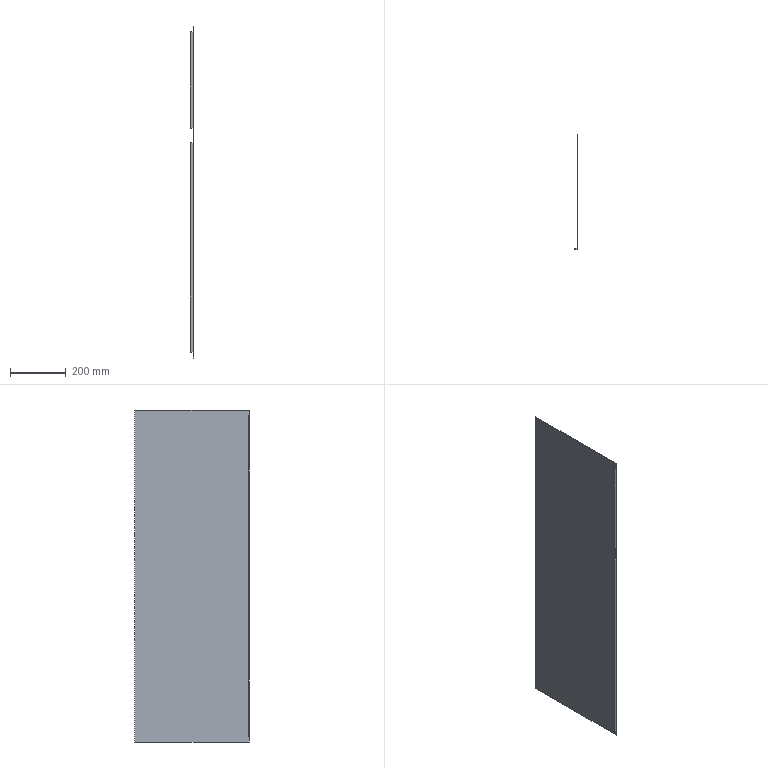Part | SolidWorks | 1 solid | 29 faces | box 12 x 410 x 1188 mm | volume 995365 mm3 | plane 27 | cylinder 2 | commonest cylinder face diameters 0.2 x1 4.2 x1
STEP:
#1=CARTESIAN_POINT('',(-2.1,-205.,176.75));
#2=VERTEX_POINT('',#1);
#3=CARTESIAN_POINT('',(-12.,-205.,176.75));
#4=VERTEX_POINT('',#3);
#5=CARTESIAN_POINT('',(-32.,-205.,176.75));
#6=DIRECTION('',(-1.,0.,0.));
#7=VECTOR('',#6,1000.);
#8=LINE('',#5,#7);
#9=EDGE_CURVE('',#2,#4,#8,.T.);
#10=ORIENTED_EDGE('',*,*,#9,.T.);
#11=CARTESIAN_POINT('',(-12.,-205.,-573.25));
#12=VERTEX_POINT('',#11);
#13=CARTESIAN_POINT('',(-12.,-205.,573.25));
#14=DIRECTION('',(0.,0.,1.));
#15=VECTOR('',#14,1000.);
#16=LINE('',#13,#15);
#17=EDGE_CURVE('',#12,#4,#16,.T.);
#18=ORIENTED_EDGE('',*,*,#17,.F.);
#19=CARTESIAN_POINT('',(-2.1,-205.,-573.25));
#20=VERTEX_POINT('',#19);
#21=CARTESIAN_POINT('',(-12.,-205.,-573.25));
#22=DIRECTION('',(-1.,0.,0.));
#23=VECTOR('',#22,1000.);
#24=LINE('',#21,#23);
#25=EDGE_CURVE('',#20,#12,#24,.T.);
#26=ORIENTED_EDGE('',*,*,#25,.F.);
#27=CARTESIAN_POINT('',(-2.1,-205.,0.));
#28=DIRECTION('',(0.,0.,1.));
#29=VECTOR('',#28,1000.);
#30=LINE('',#27,#29);
#31=EDGE_CURVE('',#20,#2,#30,.T.);
#32=ORIENTED_EDGE('',*,*,#31,.T.);
#33=EDGE_LOOP('',(#10,#18,#26,#32));
#34=FACE_OUTER_BOUND('',#33,.T.);
#35=CARTESIAN_POINT('',(0.,-205.,0.));
#36=DIRECTION('',(0.,-1.,0.));
#37=DIRECTION('',(1.,0.,0.));
#38=AXIS2_PLACEMENT_3D('',#35,#36,#37);
#39=PLANE('',#38);
#40=ADVANCED_FACE('',(#34),#39,.T.);
#41=CARTESIAN_POINT('',(-12.,-203.,-573.25));
#42=VERTEX_POINT('',#41);
#43=CARTESIAN_POINT('',(-12.,-203.,176.75));
#44=VERTEX_POINT('',#43);
#45=CARTESIAN_POINT('',(-12.,-203.,0.));
#46=DIRECTION('',(0.,0.,1.));
#47=VECTOR('',#46,1000.);
#48=LINE('',#45,#47);
#49=EDGE_CURVE('',#42,#44,#48,.T.);
#50=ORIENTED_EDGE('',*,*,#49,.T.);
#51=CARTESIAN_POINT('',(-2.1,-203.,176.75));
#52=VERTEX_POINT('',#51);
#53=CARTESIAN_POINT('',(-32.,-203.,176.75));
#54=DIRECTION('',(-1.,0.,0.));
#55=VECTOR('',#54,1000.);
#56=LINE('',#53,#55);
#57=EDGE_CURVE('',#52,#44,#56,.T.);
#58=ORIENTED_EDGE('',*,*,#57,.F.);
#59=CARTESIAN_POINT('',(-2.1,-203.,-573.25));
#60=VERTEX_POINT('',#59);
#61=CARTESIAN_POINT('',(-2.1,-203.,-573.25));
#62=DIRECTION('',(0.,0.,1.));
#63=VECTOR('',#62,1000.);
#64=LINE('',#61,#63);
#65=EDGE_CURVE('',#60,#52,#64,.T.);
#66=ORIENTED_EDGE('',*,*,#65,.F.);
#67=CARTESIAN_POINT('',(0.,-203.,-573.25));
#68=DIRECTION('',(-1.,0.,0.));
#69=VECTOR('',#68,1000.);
#70=LINE('',#67,#69);
#71=EDGE_CURVE('',#60,#42,#70,.T.);
#72=ORIENTED_EDGE('',*,*,#71,.T.);
#73=EDGE_LOOP('',(#50,#58,#66,#72));
#74=FACE_OUTER_BOUND('',#73,.T.);
#75=CARTESIAN_POINT('',(0.,-203.,0.));
#76=DIRECTION('',(0.,-1.,0.));
#77=DIRECTION('',(1.,0.,0.));
#78=AXIS2_PLACEMENT_3D('',#75,#76,#77);
#79=PLANE('',#78);
#80=ADVANCED_FACE('',(#74),#79,.F.);
#81=CARTESIAN_POINT('',(-12.,-205.001,176.75));
#82=DIRECTION('',(0.,1.,0.));
#83=VECTOR('',#82,1000.);
#84=LINE('',#81,#83);
#85=EDGE_CURVE('',#4,#44,#84,.T.);
#86=ORIENTED_EDGE('',*,*,#85,.T.);
#87=ORIENTED_EDGE('',*,*,#49,.F.);
#88=CARTESIAN_POINT('',(-12.,-205.,-573.25));
#89=DIRECTION('',(0.,1.,0.));
#90=VECTOR('',#89,1000.);
#91=LINE('',#88,#90);
#92=EDGE_CURVE('',#12,#42,#91,.T.);
#93=ORIENTED_EDGE('',*,*,#92,.F.);
#94=ORIENTED_EDGE('',*,*,#17,.T.);
#95=EDGE_LOOP('',(#86,#87,#93,#94));
#96=FACE_OUTER_BOUND('',#95,.T.);
#97=CARTESIAN_POINT('',(-12.,-205.,573.25));
#98=DIRECTION('',(-1.,0.,0.));
#99=DIRECTION('',(0.,-1.,0.));
#100=AXIS2_PLACEMENT_3D('',#97,#98,#99);
#101=PLANE('',#100);
#102=ADVANCED_FACE('',(#96),#101,.T.);
#103=CARTESIAN_POINT('',(-2.,-205.,594.25));
#104=VERTEX_POINT('',#103);
#105=CARTESIAN_POINT('',(-2.,-205.,574.25));
#106=VERTEX_POINT('',#105);
#107=CARTESIAN_POINT('',(-2.,-205.,-594.25));
#108=DIRECTION('',(0.,0.,-1.));
#109=VECTOR('',#108,1000.);
#110=LINE('',#107,#109);
#111=EDGE_CURVE('',#104,#106,#110,.T.);
#112=ORIENTED_EDGE('',*,*,#111,.T.);
#113=CARTESIAN_POINT('',(0.,-205.,574.25));
#114=VERTEX_POINT('',#113);
#115=CARTESIAN_POINT('',(-2.,-205.,574.25));
#116=DIRECTION('',(1.,0.,0.));
#117=VECTOR('',#116,1000.);
#118=LINE('',#115,#117);
#119=EDGE_CURVE('',#106,#114,#118,.T.);
#120=ORIENTED_EDGE('',*,*,#119,.T.);
#121=CARTESIAN_POINT('',(0.,-205.,594.25));
#122=VERTEX_POINT('',#121);
#123=CARTESIAN_POINT('',(0.,-205.,-594.25));
#124=DIRECTION('',(0.,0.,-1.));
#125=VECTOR('',#124,1000.);
#126=LINE('',#123,#125);
#127=EDGE_CURVE('',#122,#114,#126,.T.);
#128=ORIENTED_EDGE('',*,*,#127,.F.);
#129=CARTESIAN_POINT('',(-2.,-205.,594.25));
#130=DIRECTION('',(1.,0.,0.));
#131=VECTOR('',#130,1000.);
#132=LINE('',#129,#131);
#133=EDGE_CURVE('',#104,#122,#132,.T.);
#134=ORIENTED_EDGE('',*,*,#133,.F.);
#135=EDGE_LOOP('',(#112,#120,#128,#134));
#136=FACE_OUTER_BOUND('',#135,.T.);
#137=CARTESIAN_POINT('',(-2.,-205.,-594.25));
#138=DIRECTION('',(0.,-1.,0.));
#139=DIRECTION('',(0.,0.,-1.));
#140=AXIS2_PLACEMENT_3D('',#137,#138,#139);
#141=PLANE('',#140);
#142=ADVANCED_FACE('',(#136),#141,.T.);
#143=CARTESIAN_POINT('',(0.,-205.,-574.25));
#144=VERTEX_POINT('',#143);
#145=CARTESIAN_POINT('',(0.,-205.,-594.25));
#146=VERTEX_POINT('',#145);
#147=CARTESIAN_POINT('',(0.,-205.,-594.25));
#148=DIRECTION('',(0.,0.,-1.));
#149=VECTOR('',#148,1000.);
#150=LINE('',#147,#149);
#151=EDGE_CURVE('',#144,#146,#150,.T.);
#152=ORIENTED_EDGE('',*,*,#151,.F.);
#153=CARTESIAN_POINT('',(-2.,-205.,-574.25));
#154=VERTEX_POINT('',#153);
#155=CARTESIAN_POINT('',(-2.,-205.,-574.25));
#156=DIRECTION('',(1.,0.,0.));
#157=VECTOR('',#156,1000.);
#158=LINE('',#155,#157);
#159=EDGE_CURVE('',#154,#144,#158,.T.);
#160=ORIENTED_EDGE('',*,*,#159,.F.);
#161=CARTESIAN_POINT('',(-2.,-205.,-594.25));
#162=VERTEX_POINT('',#161);
#163=CARTESIAN_POINT('',(-2.,-205.,-594.25));
#164=DIRECTION('',(0.,0.,-1.));
#165=VECTOR('',#164,1000.);
#166=LINE('',#163,#165);
#167=EDGE_CURVE('',#154,#162,#166,.T.);
#168=ORIENTED_EDGE('',*,*,#167,.T.);
#169=CARTESIAN_POINT('',(-2.,-205.,-594.25));
#170=DIRECTION('',(1.,0.,0.));
#171=VECTOR('',#170,1000.);
#172=LINE('',#169,#171);
#173=EDGE_CURVE('',#162,#146,#172,.T.);
#174=ORIENTED_EDGE('',*,*,#173,.T.);
#175=EDGE_LOOP('',(#152,#160,#168,#174));
#176=FACE_OUTER_BOUND('',#175,.T.);
#177=CARTESIAN_POINT('',(-2.,-205.,-594.25));
#178=DIRECTION('',(0.,-1.,0.));
#179=DIRECTION('',(0.,0.,-1.));
#180=AXIS2_PLACEMENT_3D('',#177,#178,#179);
#181=PLANE('',#180);
#182=ADVANCED_FACE('',(#176),#181,.T.);
#183=CARTESIAN_POINT('',(-2.,-201.9,574.25));
#184=VERTEX_POINT('',#183);
#185=CARTESIAN_POINT('',(-2.,-205.,574.25));
#186=DIRECTION('',(0.,1.,0.));
#187=VECTOR('',#186,1000.);
#188=LINE('',#185,#187);
#189=EDGE_CURVE('',#106,#184,#188,.T.);
#190=ORIENTED_EDGE('',*,*,#189,.F.);
#191=ORIENTED_EDGE('',*,*,#111,.F.);
#192=CARTESIAN_POINT('',(-2.,205.,594.25));
#193=VERTEX_POINT('',#192);
#194=CARTESIAN_POINT('',(-2.,-205.,594.25));
#195=DIRECTION('',(0.,-1.,0.));
#196=VECTOR('',#195,1000.);
#197=LINE('',#194,#196);
#198=EDGE_CURVE('',#193,#104,#197,.T.);
#199=ORIENTED_EDGE('',*,*,#198,.F.);
#200=CARTESIAN_POINT('',(-2.,205.,-594.25));
#201=VERTEX_POINT('',#200);
#202=CARTESIAN_POINT('',(-2.,205.,-594.25));
#203=DIRECTION('',(0.,0.,1.));
#204=VECTOR('',#203,1000.);
#205=LINE('',#202,#204);
#206=EDGE_CURVE('',#201,#193,#205,.T.);
#207=ORIENTED_EDGE('',*,*,#206,.F.);
#208=CARTESIAN_POINT('',(-2.,-205.,-594.25));
#209=DIRECTION('',(0.,1.,0.));
#210=VECTOR('',#209,1000.);
#211=LINE('',#208,#210);
#212=EDGE_CURVE('',#162,#201,#211,.T.);
#213=ORIENTED_EDGE('',*,*,#212,.F.);
#214=ORIENTED_EDGE('',*,*,#167,.F.);
#215=CARTESIAN_POINT('',(-2.,-201.9,-574.25));
#216=VERTEX_POINT('',#215);
#217=CARTESIAN_POINT('',(-2.,-201.9,-574.25));
#218=DIRECTION('',(0.,-1.,0.));
#219=VECTOR('',#218,1000.);
#220=LINE('',#217,#219);
#221=EDGE_CURVE('',#216,#154,#220,.T.);
#222=ORIENTED_EDGE('',*,*,#221,.F.);
#223=CARTESIAN_POINT('',(-2.,-201.9,-573.25));
#224=VERTEX_POINT('',#223);
#225=CARTESIAN_POINT('',(-2.,-201.9,-573.25));
#226=DIRECTION('',(0.,0.,-1.));
#227=VECTOR('',#226,1000.);
#228=LINE('',#225,#227);
#229=EDGE_CURVE('',#224,#216,#228,.T.);
#230=ORIENTED_EDGE('',*,*,#229,.F.);
#231=CARTESIAN_POINT('',(-2.,-202.9,-573.25));
#232=VERTEX_POINT('',#231);
#233=CARTESIAN_POINT('',(-2.,-202.9,-573.25));
#234=DIRECTION('',(0.,1.,0.));
#235=VECTOR('',#234,1000.);
#236=LINE('',#233,#235);
#237=EDGE_CURVE('',#232,#224,#236,.T.);
#238=ORIENTED_EDGE('',*,*,#237,.F.);
#239=CARTESIAN_POINT('',(-2.,-202.9,573.25));
#240=VERTEX_POINT('',#239);
#241=CARTESIAN_POINT('',(-2.,-202.9,573.25));
#242=DIRECTION('',(0.,0.,-1.));
#243=VECTOR('',#242,1000.);
#244=LINE('',#241,#243);
#245=EDGE_CURVE('',#240,#232,#244,.T.);
#246=ORIENTED_EDGE('',*,*,#245,.F.);
#247=CARTESIAN_POINT('',(-2.,-201.9,573.25));
#248=VERTEX_POINT('',#247);
#249=CARTESIAN_POINT('',(-2.,-201.9,573.25));
#250=DIRECTION('',(0.,-1.,0.));
#251=VECTOR('',#250,1000.);
#252=LINE('',#249,#251);
#253=EDGE_CURVE('',#248,#240,#252,.T.);
#254=ORIENTED_EDGE('',*,*,#253,.F.);
#255=CARTESIAN_POINT('',(-2.,-201.9,574.25));
#256=DIRECTION('',(0.,0.,-1.));
#257=VECTOR('',#256,1000.);
#258=LINE('',#255,#257);
#259=EDGE_CURVE('',#184,#248,#258,.T.);
#260=ORIENTED_EDGE('',*,*,#259,.F.);
#261=EDGE_LOOP('',(#190,#191,#199,#207,#213,#214,#222,#230,#238,#246,#254,#260));
#262=FACE_OUTER_BOUND('',#261,.T.);
#263=CARTESIAN_POINT('',(-2.,0.,0.));
#264=DIRECTION('',(1.,0.,0.));
#265=DIRECTION('',(0.,0.,-1.));
#266=AXIS2_PLACEMENT_3D('',#263,#264,#265);
#267=PLANE('',#266);
#268=ADVANCED_FACE('',(#262),#267,.F.);
#269=ORIENTED_EDGE('',*,*,#127,.T.);
#270=CARTESIAN_POINT('',(0.,-201.9,574.25));
#271=VERTEX_POINT('',#270);
#272=CARTESIAN_POINT('',(0.,0.,574.25));
#273=DIRECTION('',(0.,1.,0.));
#274=VECTOR('',#273,1000.);
#275=LINE('',#272,#274);
#276=EDGE_CURVE('',#114,#271,#275,.T.);
#277=ORIENTED_EDGE('',*,*,#276,.T.);
#278=CARTESIAN_POINT('',(0.,-201.9,573.25));
#279=VERTEX_POINT('',#278);
#280=CARTESIAN_POINT('',(0.,-201.9,0.));
#281=DIRECTION('',(0.,0.,-1.));
#282=VECTOR('',#281,1000.);
#283=LINE('',#280,#282);
#284=EDGE_CURVE('',#271,#279,#283,.T.);
#285=ORIENTED_EDGE('',*,*,#284,.T.);
#286=CARTESIAN_POINT('',(0.,-202.9,573.25));
#287=VERTEX_POINT('',#286);
#288=CARTESIAN_POINT('',(0.,0.,573.25));
#289=DIRECTION('',(0.,-1.,0.));
#290=VECTOR('',#289,1000.);
#291=LINE('',#288,#290);
#292=EDGE_CURVE('',#279,#287,#291,.T.);
#293=ORIENTED_EDGE('',*,*,#292,.T.);
#294=CARTESIAN_POINT('',(0.,-202.9,-573.25));
#295=VERTEX_POINT('',#294);
#296=CARTESIAN_POINT('',(0.,-202.9,573.25));
#297=DIRECTION('',(0.,0.,-1.));
#298=VECTOR('',#297,1000.);
#299=LINE('',#296,#298);
#300=EDGE_CURVE('',#287,#295,#299,.T.);
#301=ORIENTED_EDGE('',*,*,#300,.T.);
#302=CARTESIAN_POINT('',(0.,-201.9,-573.25));
#303=VERTEX_POINT('',#302);
#304=CARTESIAN_POINT('',(0.,0.,-573.25));
#305=DIRECTION('',(0.,1.,0.));
#306=VECTOR('',#305,1000.);
#307=LINE('',#304,#306);
#308=EDGE_CURVE('',#295,#303,#307,.T.);
#309=ORIENTED_EDGE('',*,*,#308,.T.);
#310=CARTESIAN_POINT('',(0.,-201.9,-574.25));
#311=VERTEX_POINT('',#310);
#312=CARTESIAN_POINT('',(0.,-201.9,0.));
#313=DIRECTION('',(0.,0.,-1.));
#314=VECTOR('',#313,1000.);
#315=LINE('',#312,#314);
#316=EDGE_CURVE('',#303,#311,#315,.T.);
#317=ORIENTED_EDGE('',*,*,#316,.T.);
#318=CARTESIAN_POINT('',(0.,0.,-574.25));
#319=DIRECTION('',(0.,-1.,0.));
#320=VECTOR('',#319,1000.);
#321=LINE('',#318,#320);
#322=EDGE_CURVE('',#311,#144,#321,.T.);
#323=ORIENTED_EDGE('',*,*,#322,.T.);
#324=ORIENTED_EDGE('',*,*,#151,.T.);
#325=CARTESIAN_POINT('',(0.,205.,-594.25));
#326=VERTEX_POINT('',#325);
#327=CARTESIAN_POINT('',(0.,-205.,-594.25));
#328=DIRECTION('',(0.,1.,0.));
#329=VECTOR('',#328,1000.);
#330=LINE('',#327,#329);
#331=EDGE_CURVE('',#146,#326,#330,.T.);
#332=ORIENTED_EDGE('',*,*,#331,.T.);
#333=CARTESIAN_POINT('',(0.,205.,594.25));
#334=VERTEX_POINT('',#333);
#335=CARTESIAN_POINT('',(0.,205.,-594.25));
#336=DIRECTION('',(0.,0.,1.));
#337=VECTOR('',#336,1000.);
#338=LINE('',#335,#337);
#339=EDGE_CURVE('',#326,#334,#338,.T.);
#340=ORIENTED_EDGE('',*,*,#339,.T.);
#341=CARTESIAN_POINT('',(0.,-205.,594.25));
#342=DIRECTION('',(0.,-1.,0.));
#343=VECTOR('',#342,1000.);
#344=LINE('',#341,#343);
#345=EDGE_CURVE('',#334,#122,#344,.T.);
#346=ORIENTED_EDGE('',*,*,#345,.T.);
#347=EDGE_LOOP('',(#269,#277,#285,#293,#301,#309,#317,#323,#324,#332,#340,#346));
#348=FACE_OUTER_BOUND('',#347,.T.);
#349=CARTESIAN_POINT('',(0.,0.,0.));
#350=DIRECTION('',(1.,0.,0.));
#351=DIRECTION('',(0.,0.,-1.));
#352=AXIS2_PLACEMENT_3D('',#349,#350,#351);
#353=PLANE('',#352);
#354=ADVANCED_FACE('',(#348),#353,.T.);
#355=ORIENTED_EDGE('',*,*,#345,.F.);
#356=CARTESIAN_POINT('',(-2.,205.,594.25));
#357=DIRECTION('',(1.,0.,0.));
#358=VECTOR('',#357,1000.);
#359=LINE('',#356,#358);
#360=EDGE_CURVE('',#193,#334,#359,.T.);
#361=ORIENTED_EDGE('',*,*,#360,.F.);
#362=ORIENTED_EDGE('',*,*,#198,.T.);
#363=ORIENTED_EDGE('',*,*,#133,.T.);
#364=EDGE_LOOP('',(#355,#361,#362,#363));
#365=FACE_OUTER_BOUND('',#364,.T.);
#366=CARTESIAN_POINT('',(-2.,-205.,594.25));
#367=DIRECTION('',(0.,0.,1.));
#368=DIRECTION('',(1.,0.,0.));
#369=AXIS2_PLACEMENT_3D('',#366,#367,#368);
#370=PLANE('',#369);
#371=ADVANCED_FACE('',(#365),#370,.T.);
#372=ORIENTED_EDGE('',*,*,#339,.F.);
#373=CARTESIAN_POINT('',(-2.,205.,-594.25));
#374=DIRECTION('',(1.,0.,0.));
#375=VECTOR('',#374,1000.);
#376=LINE('',#373,#375);
#377=EDGE_CURVE('',#201,#326,#376,.T.);
#378=ORIENTED_EDGE('',*,*,#377,.F.);
#379=ORIENTED_EDGE('',*,*,#206,.T.);
#380=ORIENTED_EDGE('',*,*,#360,.T.);
#381=EDGE_LOOP('',(#372,#378,#379,#380));
#382=FACE_OUTER_BOUND('',#381,.T.);
#383=CARTESIAN_POINT('',(-2.,205.,-594.25));
#384=DIRECTION('',(0.,1.,0.));
#385=DIRECTION('',(0.,0.,1.));
#386=AXIS2_PLACEMENT_3D('',#383,#384,#385);
#387=PLANE('',#386);
#388=ADVANCED_FACE('',(#382),#387,.T.);
#389=ORIENTED_EDGE('',*,*,#331,.F.);
#390=ORIENTED_EDGE('',*,*,#173,.F.);
#391=ORIENTED_EDGE('',*,*,#212,.T.);
#392=ORIENTED_EDGE('',*,*,#377,.T.);
#393=EDGE_LOOP('',(#389,#390,#391,#392));
#394=FACE_OUTER_BOUND('',#393,.T.);
#395=CARTESIAN_POINT('',(-2.,-205.,-594.25));
#396=DIRECTION('',(0.,0.,-1.));
#397=DIRECTION('',(-1.,0.,0.));
#398=AXIS2_PLACEMENT_3D('',#395,#396,#397);
#399=PLANE('',#398);
#400=ADVANCED_FACE('',(#394),#399,.T.);
#401=ORIENTED_EDGE('',*,*,#276,.F.);
#402=ORIENTED_EDGE('',*,*,#119,.F.);
#403=ORIENTED_EDGE('',*,*,#189,.T.);
#404=CARTESIAN_POINT('',(-2.,-201.9,574.25));
#405=DIRECTION('',(1.,0.,0.));
#406=VECTOR('',#405,1000.);
#407=LINE('',#404,#406);
#408=EDGE_CURVE('',#184,#271,#407,.T.);
#409=ORIENTED_EDGE('',*,*,#408,.T.);
#410=EDGE_LOOP('',(#401,#402,#403,#409));
#411=FACE_OUTER_BOUND('',#410,.T.);
#412=CARTESIAN_POINT('',(-2.,-205.,574.25));
#413=DIRECTION('',(0.,0.,-1.));
#414=DIRECTION('',(0.,1.,0.));
#415=AXIS2_PLACEMENT_3D('',#412,#413,#414);
#416=PLANE('',#415);
#417=ADVANCED_FACE('',(#411),#416,.T.);
#418=ORIENTED_EDGE('',*,*,#284,.F.);
#419=ORIENTED_EDGE('',*,*,#408,.F.);
#420=ORIENTED_EDGE('',*,*,#259,.T.);
#421=CARTESIAN_POINT('',(-2.,-201.9,573.25));
#422=DIRECTION('',(1.,0.,0.));
#423=VECTOR('',#422,1000.);
#424=LINE('',#421,#423);
#425=EDGE_CURVE('',#248,#279,#424,.T.);
#426=ORIENTED_EDGE('',*,*,#425,.T.);
#427=EDGE_LOOP('',(#418,#419,#420,#426));
#428=FACE_OUTER_BOUND('',#427,.T.);
#429=CARTESIAN_POINT('',(-2.,-201.9,574.25));
#430=DIRECTION('',(0.,-1.,0.));
#431=DIRECTION('',(0.,0.,-1.));
#432=AXIS2_PLACEMENT_3D('',#429,#430,#431);
#433=PLANE('',#432);
#434=ADVANCED_FACE('',(#428),#433,.T.);
#435=ORIENTED_EDGE('',*,*,#292,.F.);
#436=ORIENTED_EDGE('',*,*,#425,.F.);
#437=ORIENTED_EDGE('',*,*,#253,.T.);
#438=CARTESIAN_POINT('',(-2.,-202.9,573.25));
#439=DIRECTION('',(1.,0.,0.));
#440=VECTOR('',#439,1000.);
#441=LINE('',#438,#440);
#442=EDGE_CURVE('',#240,#287,#441,.T.);
#443=ORIENTED_EDGE('',*,*,#442,.T.);
#444=EDGE_LOOP('',(#435,#436,#437,#443));
#445=FACE_OUTER_BOUND('',#444,.T.);
#446=CARTESIAN_POINT('',(-2.,-201.9,573.25));
#447=DIRECTION('',(0.,0.,1.));
#448=DIRECTION('',(1.,0.,0.));
#449=AXIS2_PLACEMENT_3D('',#446,#447,#448);
#450=PLANE('',#449);
#451=ADVANCED_FACE('',(#445),#450,.T.);
#452=ORIENTED_EDGE('',*,*,#308,.F.);
#453=CARTESIAN_POINT('',(-2.,-202.9,-573.25));
#454=DIRECTION('',(1.,0.,0.));
#455=VECTOR('',#454,1000.);
#456=LINE('',#453,#455);
#457=EDGE_CURVE('',#232,#295,#456,.T.);
#458=ORIENTED_EDGE('',*,*,#457,.F.);
#459=ORIENTED_EDGE('',*,*,#237,.T.);
#460=CARTESIAN_POINT('',(-2.,-201.9,-573.25));
#461=DIRECTION('',(1.,0.,0.));
#462=VECTOR('',#461,1000.);
#463=LINE('',#460,#462);
#464=EDGE_CURVE('',#224,#303,#463,.T.);
#465=ORIENTED_EDGE('',*,*,#464,.T.);
#466=EDGE_LOOP('',(#452,#458,#459,#465));
#467=FACE_OUTER_BOUND('',#466,.T.);
#468=CARTESIAN_POINT('',(-2.,-202.9,-573.25));
#469=DIRECTION('',(0.,0.,-1.));
#470=DIRECTION('',(-1.,0.,0.));
#471=AXIS2_PLACEMENT_3D('',#468,#469,#470);
#472=PLANE('',#471);
#473=ADVANCED_FACE('',(#467),#472,.T.);
#474=ORIENTED_EDGE('',*,*,#316,.F.);
#475=ORIENTED_EDGE('',*,*,#464,.F.);
#476=ORIENTED_EDGE('',*,*,#229,.T.);
#477=CARTESIAN_POINT('',(-2.,-201.9,-574.25));
#478=DIRECTION('',(1.,0.,0.));
#479=VECTOR('',#478,1000.);
#480=LINE('',#477,#479);
#481=EDGE_CURVE('',#216,#311,#480,.T.);
#482=ORIENTED_EDGE('',*,*,#481,.T.);
#483=EDGE_LOOP('',(#474,#475,#476,#482));
#484=FACE_OUTER_BOUND('',#483,.T.);
#485=CARTESIAN_POINT('',(-2.,-201.9,-573.25));
#486=DIRECTION('',(0.,-1.,0.));
#487=DIRECTION('',(0.,0.,-1.));
#488=AXIS2_PLACEMENT_3D('',#485,#486,#487);
#489=PLANE('',#488);
#490=ADVANCED_FACE('',(#484),#489,.T.);
#491=ORIENTED_EDGE('',*,*,#322,.F.);
#492=ORIENTED_EDGE('',*,*,#481,.F.);
#493=ORIENTED_EDGE('',*,*,#221,.T.);
#494=ORIENTED_EDGE('',*,*,#159,.T.);
#495=EDGE_LOOP('',(#491,#492,#493,#494));
#496=FACE_OUTER_BOUND('',#495,.T.);
#497=CARTESIAN_POINT('',(-2.,-201.9,-574.25));
#498=DIRECTION('',(0.,0.,1.));
#499=DIRECTION('',(1.,0.,0.));
#500=AXIS2_PLACEMENT_3D('',#497,#498,#499);
#501=PLANE('',#500);
#502=ADVANCED_FACE('',(#496),#501,.T.);
#503=CARTESIAN_POINT('',(-2.1,-205.,-573.25));
#504=DIRECTION('',(0.,-1.,0.));
#505=VECTOR('',#504,1000.);
#506=LINE('',#503,#505);
#507=EDGE_CURVE('',#60,#20,#506,.T.);
#508=ORIENTED_EDGE('',*,*,#507,.F.);
#509=CARTESIAN_POINT('',(-2.1,-202.9,-573.25));
#510=DIRECTION('',(0.,0.,-1.));
#511=DIRECTION('',(1.,0.,0.));
#512=AXIS2_PLACEMENT_3D('',#509,#510,#511);
#513=CIRCLE('',#512,0.1);
#514=EDGE_CURVE('',#232,#60,#513,.T.);
#515=ORIENTED_EDGE('',*,*,#514,.F.);
#516=ORIENTED_EDGE('',*,*,#457,.T.);
#517=CARTESIAN_POINT('',(-2.1,-202.9,-573.25));
#518=DIRECTION('',(0.,0.,-1.));
#519=DIRECTION('',(1.,0.,0.));
#520=AXIS2_PLACEMENT_3D('',#517,#518,#519);
#521=CIRCLE('',#520,2.1);
#522=EDGE_CURVE('',#295,#20,#521,.T.);
#523=ORIENTED_EDGE('',*,*,#522,.T.);
#524=EDGE_LOOP('',(#508,#515,#516,#523));
#525=FACE_OUTER_BOUND('',#524,.T.);
#526=CARTESIAN_POINT('',(-2.1,-202.9,-573.25));
#527=DIRECTION('',(0.,0.,-1.));
#528=DIRECTION('',(-1.,0.,0.));
#529=AXIS2_PLACEMENT_3D('',#526,#527,#528);
#530=PLANE('',#529);
#531=ADVANCED_FACE('',(#525),#530,.T.);
#532=CARTESIAN_POINT('',(-2.1,-203.,573.25));
#533=VERTEX_POINT('',#532);
#534=CARTESIAN_POINT('',(-2.1,-202.9,573.25));
#535=DIRECTION('',(0.,0.,1.));
#536=DIRECTION('',(1.,0.,0.));
#537=AXIS2_PLACEMENT_3D('',#534,#535,#536);
#538=CIRCLE('',#537,0.1);
#539=EDGE_CURVE('',#533,#240,#538,.T.);
#540=ORIENTED_EDGE('',*,*,#539,.F.);
#541=CARTESIAN_POINT('',(-2.1,-205.,573.25));
#542=VERTEX_POINT('',#541);
#543=CARTESIAN_POINT('',(-2.1,-203.,573.25));
#544=DIRECTION('',(0.,-1.,0.));
#545=VECTOR('',#544,1000.);
#546=LINE('',#543,#545);
#547=EDGE_CURVE('',#533,#542,#546,.T.);
#548=ORIENTED_EDGE('',*,*,#547,.T.);
#549=CARTESIAN_POINT('',(-2.1,-202.9,573.25));
#550=DIRECTION('',(0.,0.,1.));
#551=DIRECTION('',(1.,0.,0.));
#552=AXIS2_PLACEMENT_3D('',#549,#550,#551);
#553=CIRCLE('',#552,2.1);
#554=EDGE_CURVE('',#542,#287,#553,.T.);
#555=ORIENTED_EDGE('',*,*,#554,.T.);
#556=ORIENTED_EDGE('',*,*,#442,.F.);
#557=EDGE_LOOP('',(#540,#548,#555,#556));
#558=FACE_OUTER_BOUND('',#557,.T.);
#559=CARTESIAN_POINT('',(-2.1,-202.9,573.25));
#560=DIRECTION('',(0.,0.,-1.));
#561=DIRECTION('',(-1.,0.,0.));
#562=AXIS2_PLACEMENT_3D('',#559,#560,#561);
#563=PLANE('',#562);
#564=ADVANCED_FACE('',(#558),#563,.F.);
#565=CARTESIAN_POINT('',(-2.,-204.998,176.75));
#566=VERTEX_POINT('',#565);
#567=CARTESIAN_POINT('',(-2.1,-202.9,176.75));
#568=DIRECTION('',(0.,0.,-1.));
#569=DIRECTION('',(0.,1.,0.));
#570=AXIS2_PLACEMENT_3D('',#567,#568,#569);
#571=CIRCLE('',#570,2.1);
#572=EDGE_CURVE('',#566,#2,#571,.T.);
#573=ORIENTED_EDGE('',*,*,#572,.T.);
#574=ORIENTED_EDGE('',*,*,#31,.F.);
#575=ORIENTED_EDGE('',*,*,#522,.F.);
#576=ORIENTED_EDGE('',*,*,#300,.F.);
#577=ORIENTED_EDGE('',*,*,#554,.F.);
#578=CARTESIAN_POINT('',(-2.1,-205.,228.75));
#579=VERTEX_POINT('',#578);
#580=CARTESIAN_POINT('',(-2.1,-205.,0.));
#581=DIRECTION('',(0.,0.,1.));
#582=VECTOR('',#581,1000.);
#583=LINE('',#580,#582);
#584=EDGE_CURVE('',#579,#542,#583,.T.);
#585=ORIENTED_EDGE('',*,*,#584,.F.);
#586=CARTESIAN_POINT('',(-2.,-204.998,228.75));
#587=VERTEX_POINT('',#586);
#588=CARTESIAN_POINT('',(-2.1,-202.9,228.75));
#589=DIRECTION('',(0.,0.,1.));
#590=DIRECTION('',(1.,0.,0.));
#591=AXIS2_PLACEMENT_3D('',#588,#589,#590);
#592=CIRCLE('',#591,2.1);
#593=EDGE_CURVE('',#579,#587,#592,.T.);
#594=ORIENTED_EDGE('',*,*,#593,.T.);
#595=CARTESIAN_POINT('',(-2.,-204.998,573.25));
#596=DIRECTION('',(0.,0.,-1.));
#597=VECTOR('',#596,1000.);
#598=LINE('',#595,#597);
#599=EDGE_CURVE('',#587,#566,#598,.T.);
#600=ORIENTED_EDGE('',*,*,#599,.T.);
#601=EDGE_LOOP('',(#573,#574,#575,#576,#577,#585,#594,#600));
#602=FACE_OUTER_BOUND('',#601,.T.);
#603=CARTESIAN_POINT('',(-2.1,-202.9,573.25));
#604=DIRECTION('',(0.,0.,1.));
#605=DIRECTION('',(0.,-1.,0.));
#606=AXIS2_PLACEMENT_3D('',#603,#604,#605);
#607=CYLINDRICAL_SURFACE('',#606,2.1);
#608=ADVANCED_FACE('',(#602),#607,.T.);
#609=ORIENTED_EDGE('',*,*,#245,.T.);
#610=ORIENTED_EDGE('',*,*,#514,.T.);
#611=ORIENTED_EDGE('',*,*,#65,.T.);
#612=CARTESIAN_POINT('',(-2.1,-203.,228.75));
#613=VERTEX_POINT('',#612);
#614=CARTESIAN_POINT('',(-2.1,-203.,573.25));
#615=DIRECTION('',(0.,0.,-1.));
#616=VECTOR('',#615,1000.);
#617=LINE('',#614,#616);
#618=EDGE_CURVE('',#613,#52,#617,.T.);
#619=ORIENTED_EDGE('',*,*,#618,.F.);
#620=CARTESIAN_POINT('',(-2.1,-203.,-573.25));
#621=DIRECTION('',(0.,0.,1.));
#622=VECTOR('',#621,1000.);
#623=LINE('',#620,#622);
#624=EDGE_CURVE('',#613,#533,#623,.T.);
#625=ORIENTED_EDGE('',*,*,#624,.T.);
#626=ORIENTED_EDGE('',*,*,#539,.T.);
#627=EDGE_LOOP('',(#609,#610,#611,#619,#625,#626));
#628=FACE_OUTER_BOUND('',#627,.T.);
#629=CARTESIAN_POINT('',(-2.1,-202.9,573.25));
#630=DIRECTION('',(0.,0.,1.));
#631=DIRECTION('',(0.,-1.,0.));
#632=AXIS2_PLACEMENT_3D('',#629,#630,#631);
#633=CYLINDRICAL_SURFACE('',#632,0.1);
#634=ADVANCED_FACE('',(#628),#633,.F.);
#635=CARTESIAN_POINT('',(-12.,-205.,573.25));
#636=VERTEX_POINT('',#635);
#637=CARTESIAN_POINT('',(-2.,-205.,573.25));
#638=DIRECTION('',(1.,0.,0.));
#639=VECTOR('',#638,1000.);
#640=LINE('',#637,#639);
#641=EDGE_CURVE('',#636,#542,#640,.T.);
#642=ORIENTED_EDGE('',*,*,#641,.T.);
#643=ORIENTED_EDGE('',*,*,#547,.F.);
#644=CARTESIAN_POINT('',(-12.,-203.,573.25));
#645=VERTEX_POINT('',#644);
#646=CARTESIAN_POINT('',(0.,-203.,573.25));
#647=DIRECTION('',(1.,0.,0.));
#648=VECTOR('',#647,1000.);
#649=LINE('',#646,#648);
#650=EDGE_CURVE('',#645,#533,#649,.T.);
#651=ORIENTED_EDGE('',*,*,#650,.F.);
#652=CARTESIAN_POINT('',(-12.,-205.,573.25));
#653=DIRECTION('',(0.,1.,0.));
#654=VECTOR('',#653,1000.);
#655=LINE('',#652,#654);
#656=EDGE_CURVE('',#636,#645,#655,.T.);
#657=ORIENTED_EDGE('',*,*,#656,.F.);
#658=EDGE_LOOP('',(#642,#643,#651,#657));
#659=FACE_OUTER_BOUND('',#658,.T.);
#660=CARTESIAN_POINT('',(-2.,-205.,573.25));
#661=DIRECTION('',(0.,0.,1.));
#662=DIRECTION('',(0.,-1.,0.));
#663=AXIS2_PLACEMENT_3D('',#660,#661,#662);
#664=PLANE('',#663);
#665=ADVANCED_FACE('',(#659),#664,.T.);
#666=ORIENTED_EDGE('',*,*,#71,.F.);
#667=ORIENTED_EDGE('',*,*,#507,.T.);
#668=ORIENTED_EDGE('',*,*,#25,.T.);
#669=ORIENTED_EDGE('',*,*,#92,.T.);
#670=EDGE_LOOP('',(#666,#667,#668,#669));
#671=FACE_OUTER_BOUND('',#670,.T.);
#672=CARTESIAN_POINT('',(-12.,-205.,-573.25));
#673=DIRECTION('',(0.,0.,-1.));
#674=DIRECTION('',(-1.,0.,0.));
#675=AXIS2_PLACEMENT_3D('',#672,#673,#674);
#676=PLANE('',#675);
#677=ADVANCED_FACE('',(#671),#676,.T.);
#678=CARTESIAN_POINT('',(-12.,-205.,228.75));
#679=VERTEX_POINT('',#678);
#680=CARTESIAN_POINT('',(-32.,-205.,228.75));
#681=DIRECTION('',(1.,0.,0.));
#682=VECTOR('',#681,1000.);
#683=LINE('',#680,#682);
#684=EDGE_CURVE('',#679,#579,#683,.T.);
#685=ORIENTED_EDGE('',*,*,#684,.T.);
#686=ORIENTED_EDGE('',*,*,#584,.T.);
#687=ORIENTED_EDGE('',*,*,#641,.F.);
#688=CARTESIAN_POINT('',(-12.,-205.,573.25));
#689=DIRECTION('',(0.,0.,1.));
#690=VECTOR('',#689,1000.);
#691=LINE('',#688,#690);
#692=EDGE_CURVE('',#679,#636,#691,.T.);
#693=ORIENTED_EDGE('',*,*,#692,.F.);
#694=EDGE_LOOP('',(#685,#686,#687,#693));
#695=FACE_OUTER_BOUND('',#694,.T.);
#696=CARTESIAN_POINT('',(0.,-205.,0.));
#697=DIRECTION('',(0.,-1.,0.));
#698=DIRECTION('',(1.,0.,0.));
#699=AXIS2_PLACEMENT_3D('',#696,#697,#698);
#700=PLANE('',#699);
#701=ADVANCED_FACE('',(#695),#700,.T.);
#702=ORIENTED_EDGE('',*,*,#624,.F.);
#703=CARTESIAN_POINT('',(-12.,-203.,228.75));
#704=VERTEX_POINT('',#703);
#705=CARTESIAN_POINT('',(-32.,-203.,228.75));
#706=DIRECTION('',(1.,0.,0.));
#707=VECTOR('',#706,1000.);
#708=LINE('',#705,#707);
#709=EDGE_CURVE('',#704,#613,#708,.T.);
#710=ORIENTED_EDGE('',*,*,#709,.F.);
#711=CARTESIAN_POINT('',(-12.,-203.,0.));
#712=DIRECTION('',(0.,0.,1.));
#713=VECTOR('',#712,1000.);
#714=LINE('',#711,#713);
#715=EDGE_CURVE('',#704,#645,#714,.T.);
#716=ORIENTED_EDGE('',*,*,#715,.T.);
#717=ORIENTED_EDGE('',*,*,#650,.T.);
#718=EDGE_LOOP('',(#702,#710,#716,#717));
#719=FACE_OUTER_BOUND('',#718,.T.);
#720=CARTESIAN_POINT('',(0.,-203.,0.));
#721=DIRECTION('',(0.,-1.,0.));
#722=DIRECTION('',(1.,0.,0.));
#723=AXIS2_PLACEMENT_3D('',#720,#721,#722);
#724=PLANE('',#723);
#725=ADVANCED_FACE('',(#719),#724,.F.);
#726=CARTESIAN_POINT('',(-12.,-205.001,228.75));
#727=DIRECTION('',(0.,-1.,0.));
#728=VECTOR('',#727,1000.);
#729=LINE('',#726,#728);
#730=EDGE_CURVE('',#704,#679,#729,.T.);
#731=ORIENTED_EDGE('',*,*,#730,.T.);
#732=ORIENTED_EDGE('',*,*,#692,.T.);
#733=ORIENTED_EDGE('',*,*,#656,.T.);
#734=ORIENTED_EDGE('',*,*,#715,.F.);
#735=EDGE_LOOP('',(#731,#732,#733,#734));
#736=FACE_OUTER_BOUND('',#735,.T.);
#737=CARTESIAN_POINT('',(-12.,-205.,573.25));
#738=DIRECTION('',(-1.,0.,0.));
#739=DIRECTION('',(0.,-1.,0.));
#740=AXIS2_PLACEMENT_3D('',#737,#738,#739);
#741=PLANE('',#740);
#742=ADVANCED_FACE('',(#736),#741,.T.);
#743=CARTESIAN_POINT('',(-2.,-203.,176.75));
#744=VERTEX_POINT('',#743);
#745=CARTESIAN_POINT('',(-2.,-205.001,176.75));
#746=DIRECTION('',(0.,1.,0.));
#747=VECTOR('',#746,1000.);
#748=LINE('',#745,#747);
#749=EDGE_CURVE('',#566,#744,#748,.T.);
#750=ORIENTED_EDGE('',*,*,#749,.T.);
#751=CARTESIAN_POINT('',(-32.,-203.,176.75));
#752=DIRECTION('',(-1.,0.,0.));
#753=VECTOR('',#752,1000.);
#754=LINE('',#751,#753);
#755=EDGE_CURVE('',#744,#52,#754,.T.);
#756=ORIENTED_EDGE('',*,*,#755,.T.);
#757=ORIENTED_EDGE('',*,*,#57,.T.);
#758=ORIENTED_EDGE('',*,*,#85,.F.);
#759=ORIENTED_EDGE('',*,*,#9,.F.);
#760=ORIENTED_EDGE('',*,*,#572,.F.);
#761=EDGE_LOOP('',(#750,#756,#757,#758,#759,#760));
#762=FACE_OUTER_BOUND('',#761,.T.);
#763=CARTESIAN_POINT('',(-32.,-205.001,176.75));
#764=DIRECTION('',(0.,0.,-1.));
#765=DIRECTION('',(0.,1.,0.));
#766=AXIS2_PLACEMENT_3D('',#763,#764,#765);
#767=PLANE('',#766);
#768=ADVANCED_FACE('',(#762),#767,.F.);
#769=CARTESIAN_POINT('',(-2.,-203.,228.75));
#770=VERTEX_POINT('',#769);
#771=CARTESIAN_POINT('',(-2.,-205.001,228.75));
#772=DIRECTION('',(0.,1.,0.));
#773=VECTOR('',#772,1000.);
#774=LINE('',#771,#773);
#775=EDGE_CURVE('',#587,#770,#774,.T.);
#776=ORIENTED_EDGE('',*,*,#775,.T.);
#777=CARTESIAN_POINT('',(-2.,-203.,176.75));
#778=DIRECTION('',(0.,0.,-1.));
#779=VECTOR('',#778,1000.);
#780=LINE('',#777,#779);
#781=EDGE_CURVE('',#770,#744,#780,.T.);
#782=ORIENTED_EDGE('',*,*,#781,.T.);
#783=ORIENTED_EDGE('',*,*,#749,.F.);
#784=ORIENTED_EDGE('',*,*,#599,.F.);
#785=EDGE_LOOP('',(#776,#782,#783,#784));
#786=FACE_OUTER_BOUND('',#785,.T.);
#787=CARTESIAN_POINT('',(-2.,-205.001,176.75));
#788=DIRECTION('',(1.,0.,0.));
#789=DIRECTION('',(0.,1.,0.));
#790=AXIS2_PLACEMENT_3D('',#787,#788,#789);
#791=PLANE('',#790);
#792=ADVANCED_FACE('',(#786),#791,.F.);
#793=ORIENTED_EDGE('',*,*,#684,.F.);
#794=ORIENTED_EDGE('',*,*,#730,.F.);
#795=ORIENTED_EDGE('',*,*,#709,.T.);
#796=CARTESIAN_POINT('',(-32.,-203.,228.75));
#797=DIRECTION('',(1.,0.,0.));
#798=VECTOR('',#797,1000.);
#799=LINE('',#796,#798);
#800=EDGE_CURVE('',#613,#770,#799,.T.);
#801=ORIENTED_EDGE('',*,*,#800,.T.);
#802=ORIENTED_EDGE('',*,*,#775,.F.);
#803=ORIENTED_EDGE('',*,*,#593,.F.);
#804=EDGE_LOOP('',(#793,#794,#795,#801,#802,#803));
#805=FACE_OUTER_BOUND('',#804,.T.);
#806=CARTESIAN_POINT('',(-32.,-205.001,228.75));
#807=DIRECTION('',(0.,0.,1.));
#808=DIRECTION('',(1.,0.,0.));
#809=AXIS2_PLACEMENT_3D('',#806,#807,#808);
#810=PLANE('',#809);
#811=ADVANCED_FACE('',(#805),#810,.F.);
#812=ORIENTED_EDGE('',*,*,#618,.T.);
#813=ORIENTED_EDGE('',*,*,#755,.F.);
#814=ORIENTED_EDGE('',*,*,#781,.F.);
#815=ORIENTED_EDGE('',*,*,#800,.F.);
#816=EDGE_LOOP('',(#812,#813,#814,#815));
#817=FACE_OUTER_BOUND('',#816,.T.);
#818=CARTESIAN_POINT('',(0.,-203.,0.));
#819=DIRECTION('',(0.,1.,0.));
#820=DIRECTION('',(-1.,0.,0.));
#821=AXIS2_PLACEMENT_3D('',#818,#819,#820);
#822=PLANE('',#821);
#823=ADVANCED_FACE('',(#817),#822,.F.);
#824=CLOSED_SHELL('',(#40,#80,#102,#142,#182,#268,#354,#371,#388,#400,#417,#434,#451,#473,#490,#502,#531,#564,#608,#634,#665,#677,#701,#725,#742,#768,#792,#811,#823));
#825=MANIFOLD_SOLID_BREP('',#824);
#826=CARTESIAN_POINT('',(0.,0.,0.));
#827=DIRECTION('',(0.,0.,1.));
#828=DIRECTION('',(1.,0.,0.));
#829=AXIS2_PLACEMENT_3D('',#826,#827,#828);
#830=(LENGTH_UNIT()NAMED_UNIT(*)SI_UNIT(.MILLI.,.METRE.));
#831=UNCERTAINTY_MEASURE_WITH_UNIT(LENGTH_MEASURE(0.00001),#830,'','');
#832=(NAMED_UNIT(*)PLANE_ANGLE_UNIT()SI_UNIT($,.RADIAN.));
#833=(NAMED_UNIT(*)SI_UNIT($,.STERADIAN.)SOLID_ANGLE_UNIT());
#834=(GEOMETRIC_REPRESENTATION_CONTEXT(3)GLOBAL_UNCERTAINTY_ASSIGNED_CONTEXT((#831))GLOBAL_UNIT_ASSIGNED_CONTEXT((#830,#832,#833))REPRESENTATION_CONTEXT('',''));
#835=ADVANCED_BREP_SHAPE_REPRESENTATION('',(#825,#829),#834);